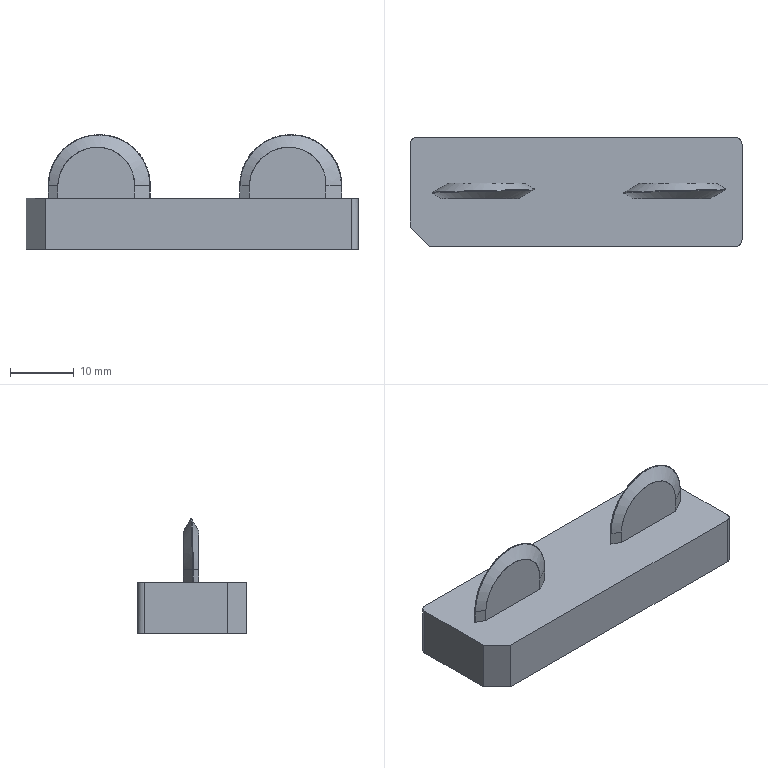NC program | PowerMill | posted with a generic post | part box 52 x 17 x 17.993 mm
Lines 1 to 1042 of 175197:
%
O0001
N104 ( POWERMILL CB  : 2026004.0)
N105 ( POST VER      : 2026.0.0.5161)
N106 ( OPTION FILE   : FANUC)
N107 ( OUTPUT WORKPLANE : WORLD)
N108 (  )
N109 ( TOOL LIST )
N110 (---------------------------------------)
N111 ( NO. | ID        | DIA.| TIP RAD|LENGTH)
N112 (---------------------------------------)
N113 (    1|D10C_1_1_1 |10.0 |  0.0   |73.44 )
N114 (    2|D4C_1_1    | 4.0 |  0.0   |65.16 )
N115 (    3|D10_1_1_1  |10.0 |  0.0   |73.16 )
N116 (    4|R1_1_1     | 2.0 |  1.0   | 64.4 )
N117 (   10|D3_1_1     | 3.0 |  0.0   |65.28 )
N118 (   13|TEXT_D4_1_1| 4.0 |  0.3   |65.24 )
N119 (---------------------------------------)
N120 (  )
N121 ( NUMBER OF TOOLPATHS: 9.0 )
N122 ( ESTIMATED PROGRAM DURATION: 0 HOURS 14 MIN 44 SEC)
N123 (  )
N124 G00 G21 G80 G40 G17
N125 G90
N126 G54
N127 G53 Z0.0
N128 (---------------)
N129 ( START TOOLPATH : 精公开粗01-扫面平行-D10C )
N130 (---------------)
N131 ( TOOL NO.    :1 )
N132 ( TOOL TYPE   : ENDMILL)
N133 ( TOOL ID     : D10C_1_1_1)
N134 ( TOOL DIA    : 10.0 LENGTH 73.44)
N135 T1
N136 M6
N137 S8000 M03
N138 G00 G90 X0.0 Y0.0
N139 G43 Z10.2 H1
N140
N141 G05 P10000 R4
N142 X33.8 Y11.3
N143 Z1.152
N144 G01 Z-0.048 F6000.0
N145 X28.8 F10000.0
N146 X-28.8
N147 Y5.65
N148 X28.8
N149 Y0.0
N150 X-28.8
N151 Y-5.65
N152 X28.8
N153 Y-11.3
N154 X-28.8
N155 X-33.8
N156 G00 Z10.2
N157 G05 P0
N158 (---------------)
N159 ( END TOOLPATH : 精公开粗01-扫面平行-D10C )
N160 (---------------)
N161 ( START TOOLPATH : 精公开粗01-外形偏置-D10C )
N162 (---------------)
N163 G00 X0.467 Y0.0 Z9.902
N164 G05 P10000 R4
N165 X-20.1146 Y16.575
N166 Z0.7059
N167 G01 Z-0.4941 F6000.0
N168 Y16.0475 F10000.0
N169 G03 X-15.3671 Y11.3 I4.7475 J0.0
N170 G01 X15.031
N171 X15.3555 Y5.6619
N172 X15.5488 Y5.6731
N173 X16.3222 Y5.6668
N174 X17.8691 Y5.5575
N175 X18.6425 Y5.4508
N176 X19.4159 Y5.2563
N177 X20.1894 Y4.9472
N178 X20.9628 Y4.4839
N179 X21.2604 Y4.2538
N180 X21.7362 Y3.8022
N181 X22.0145 Y3.4804
N182 X22.5239 Y2.707
N183 X22.8623 Y1.9336
N184 X23.0648 Y1.1601
N185 X23.1469 Y0.3867
N186 X23.1193 Y-0.3867
N187 X22.9748 Y-1.1601
N188 X22.7059 Y-1.9336
N189 X22.5097 Y-2.3365
N190 X22.2861 Y-2.707
N191 X21.7362 Y-3.4106
N192 X20.9628 Y-4.0912
N193 X20.7243 Y-4.2538
N194 X20.1894 Y-4.5543
N195 X19.4159 Y-4.8679
N196 X18.8482 Y-5.0273
N197 X17.8691 Y-5.1979
N198 X16.3222 Y-5.3576
N199 X15.5488 Y-5.3924
N200 X14.7754 Y-5.3899
N201 X13.2285 Y-5.2939
N202 X12.4551 Y-5.198
N203 X11.699 Y-5.0273
N204 X10.9083 Y-4.739
N205 X10.1348 Y-4.3084
N206 X9.3614 Y-3.6778
N207 X9.1718 Y-3.4804
N208 X8.5866 Y-2.707
N209 X8.1955 Y-1.9336
N210 X7.9426 Y-1.1601
N211 X7.8191 Y-0.3867
N212 X7.813 Y0.0303
N213 X3.1961 Y-0.0196
N214 G03 X3.8356 Y-3.4017 I9.825 J0.1062
N215 G01 X4.3225 Y-4.6838
N216 G02 X2.9383 Y-6.6901 I-1.3842 J-0.5257
N217 G01 X-2.0806 Y-6.6902
N218 G02 X-3.432 Y-4.7024 I0.0 J1.4533
N219 G01 X-2.9405 Y-3.4598
N220 G03 X-2.4579 Y-1.8025 I-8.6123 J3.4066
N221 G01 X-2.4294 Y-1.6543
N222 G03 X-2.7691 Y3.3599 I-9.6844 J1.8626
N223 G01 X-3.2133 Y4.677
N224 G02 X-1.7677 Y6.6901 I1.4456 J0.4875
N225 G01 X2.808
N226 G02 X4.2262 Y4.6814 I0.0 J-1.505
N227 G01 X3.7623 Y3.3756
N228 G03 X3.1961 Y-0.0196 I9.2588 J-3.289
N229 G01 X7.813 Y0.0303
N230 X7.8079 Y0.3867
N231 X7.9066 Y1.1601
N232 X8.1281 Y1.9336
N233 X8.4898 Y2.707
N234 X9.0292 Y3.4804
N235 X9.3614 Y3.8391
N236 X9.8321 Y4.2538
N237 X10.1348 Y4.4713
N238 X10.9083 Y4.9014
N239 X11.6817 Y5.1919
N240 X12.4551 Y5.3725
N241 X13.2285 Y5.4966
N242 X14.002 Y5.584
N243 X15.3555 Y5.6619
N244 X15.031 Y11.3
N245 X30.256
N246 G02 X31.256 Y10.3 I0.0 J-1.0
N247 G01 Y6.2153
N248 X26.256
N249 Y6.1307
N250 X26.1901 Y6.2308
N251 X26.167 Y6.2655
N252 X26.1436 Y6.3
N253 X26.256
N254 Y6.2153
N255 X31.256
N256 Y-6.1354
N257 X26.3408
N258 G02 X25.9821 I-0.1793 J0.0
N259 G02 X26.3408 I0.1794 J0.0
N260 G01 X31.256
N261 Y-10.3
N262 G02 X30.256 Y-11.3 I-1.0 J0.0
N263 G01 X-29.322
N264 G02 X-30.322 Y-10.3 I0.0 J1.0
N265 G01 Y10.3
N266 G02 X-29.322 Y11.3 I1.0 J0.0
N267 G01 X-25.2388
N268 Y6.3515
N269 G02 X-25.1309 Y6.2436 I0.0 J-0.1079
N270 G02 X-25.3467 I-0.1079 J0.0
N271 G02 X-25.2388 Y6.3515 I0.1079 J0.0
N272 G01 Y11.3
N273 X-15.3671
N274 X-15.0982 Y5.6473
N275 X-14.6148 Y5.6703
N276 X-13.8414 Y5.6695
N277 X-12.2945 Y5.5758
N278 X-11.5211 Y5.4789
N279 X-10.7477 Y5.3053
N280 X-9.9743 Y5.0224
N281 X-9.2008 Y4.5959
N282 X-8.7397 Y4.2538
N283 X-8.4274 Y3.9714
N284 X-7.9851 Y3.4804
N285 X-7.654 Y3.0059
N286 X-7.4764 Y2.707
N287 X-7.1374 Y1.9336
N288 X-6.9344 Y1.1601
N289 X-6.8536 Y0.3867
N290 X-6.8804 Y-0.3867
N291 X-7.0249 Y-1.1601
N292 X-7.2911 Y-1.9336
N293 X-7.654 Y-2.6161
N294 X-8.33 Y-3.4804
N295 X-9.2008 Y-4.2047
N296 X-9.9743 Y-4.6313
N297 X-10.7477 Y-4.9196
N298 X-11.1518 Y-5.0273
N299 X-12.2945 Y-5.2213
N300 X-13.8414 Y-5.3676
N301 X-14.6148 Y-5.3932
N302 X-15.3882 Y-5.3883
N303 X-16.9351 Y-5.2745
N304 X-17.7085 Y-5.1703
N305 X-18.3007 Y-5.0273
N306 X-19.2554 Y-4.6605
N307 X-19.9459 Y-4.2538
N308 X-20.8022 Y-3.5089
N309 X-21.0038 Y-3.2441
N310 X-25.1615 Y-6.1065
N311 X-25.1581 Y-6.112
N312 X-25.1552 Y-6.1179
N313 X-25.1337 Y-6.1686
N314 G02 X-25.2221 Y-6.2283 I-0.05 J-0.0213
N315 G01 X-25.2363 Y-6.2142
N316 X-25.2611 Y-6.1893
N317 X-25.2798 Y-6.1371
N318 X-25.2514 Y-6.0894
N319 X-25.203 Y-6.0795
N320 X-25.1615 Y-6.1065
N321 X-21.0038 Y-3.2441
N322 X-21.4128 Y-2.707
N323 X-21.5757 Y-2.4236
N324 X-21.8083 Y-1.9336
N325 X-22.0574 Y-1.1601
N326 X-22.1813 Y-0.3867
N327 X-22.1923 Y0.3867
N328 X-22.0932 Y1.1601
N329 X-21.8712 Y1.9336
N330 X-21.5757 Y2.584
N331 X-20.9712 Y3.4804
N332 X-20.8022 Y3.6702
N333 X-20.1679 Y4.2538
N334 X-19.2554 Y4.8241
N335 X-18.4819 Y5.1405
N336 X-17.7085 Y5.343
N337 X-16.9351 Y5.4724
N338 X-15.3882 Y5.6335
N339 X-15.0982 Y5.6473
N340 X-15.3671 Y11.3
N341 G00 Z3.3098
N342 G01 X-20.1146 Y16.575
N343 G00 Z0.3098
N344 G01 Z-0.8902 F6000.0
N345 Y16.0475 F10000.0
N346 G03 X-15.3671 Y11.3 I4.7475 J0.0
N347 G01 X14.5559
N348 X14.7754 Y5.8707
N349 X15.5488 Y5.9019
N350 X16.3222 Y5.8955
N351 X17.692 Y5.8007
N352 X18.6425 Y5.6777
N353 X19.4159 Y5.5428
N354 X20.1894 Y5.369
N355 X20.9628 Y5.0864
N356 X21.7362 Y4.6711
N357 X22.299 Y4.2538
N358 X22.5097 Y4.0648
N359 X23.0411 Y3.4804
N360 X23.2831 Y3.1445
N361 X23.5417 Y2.707
N362 X23.8766 Y1.9336
N363 X24.0565 Y1.2516
N364 X24.1504 Y0.3867
N365 X24.1217 Y-0.3867
N366 X24.0565 Y-0.8111
N367 X23.9729 Y-1.1601
N368 X23.7015 Y-1.9336
N369 X23.2831 Y-2.6992
N370 X22.6539 Y-3.4804
N371 X22.5097 Y-3.6199
N372 X21.7362 Y-4.2297
N373 X20.9628 Y-4.6486
N374 X20.1894 Y-4.9331
N375 X19.8327 Y-5.0273
N376 X18.6425 Y-5.2871
N377 X17.8691 Y-5.4178
N378 X16.3222 Y-5.5853
N379 X15.5488 Y-5.6207
N380 X14.7754 Y-5.6194
N381 X14.002 Y-5.5836
N382 X12.4551 Y-5.4231
N383 X10.9083 Y-5.1305
N384 X10.5494 Y-5.0273
N385 X10.1348 Y-4.8727
N386 X9.3614 Y-4.4858
N387 X9.0092 Y-4.2538
N388 X8.588 Y-3.9225
N389 X8.1409 Y-3.4804
N390 X7.8146 Y-3.0792
N391 X7.5656 Y-2.707
N392 X7.1758 Y-1.9336
N393 X6.9324 Y-1.1601
N394 X6.8121 Y-0.3867
N395 X6.8044 Y0.3867
N396 X6.9081 Y1.1601
N397 X7.0411 Y1.6716
N398 X7.1333 Y1.9336
N399 X7.4984 Y2.707
N400 X7.8146 Y3.1908
N401 X8.042 Y3.4804
N402 X8.588 Y4.036
N403 X8.8527 Y4.2538
N404 X9.3614 Y4.5993
N405 X10.1348 Y4.9913
N406 X10.9083 Y5.2519
N407 X12.4551 Y5.5906
N408 X13.2285 Y5.7174
N409 X14.7754 Y5.8707
N410 X14.5559 Y11.3
N411 X30.256
N412 G02 X31.256 Y10.3 I0.0 J-1.0
N413 G01 Y-10.3
N414 G02 X30.256 Y-11.3 I-1.0 J0.0
N415 G01 X-29.322
N416 G02 X-30.322 Y-10.3 I0.0 J1.0
N417 G01 Y10.3
N418 G02 X-29.322 Y11.3 I1.0 J0.0
N419 G01 X-15.6424
N420 X-15.3882 Y5.8625
N421 X-14.6148 Y5.8986
N422 X-13.8414 Y5.8987
N423 X-12.2945 Y5.7998
N424 X-11.5211 Y5.7026
N425 X-9.9743 Y5.4127
N426 X-9.2008 Y5.1556
N427 X-8.9067 Y5.0273
N428 X-8.4274 Y4.773
N429 X-7.7017 Y4.2538
N430 X-6.9595 Y3.4804
N431 X-6.4581 Y2.707
N432 X-6.1243 Y1.9336
N433 X-5.9279 Y1.1601
N434 X-5.8479 Y0.3867
N435 X-5.859 Y0.1083
N436 X-0.0971 Y-0.0337
N437 G03 X-0.4974 Y3.175 I-10.9069 J0.2687
N438 G01 X-0.7678 Y4.1414
N439 G02 X0.3038 Y5.554 I1.0716 J0.2999
N440 G01 X0.7376
N441 G02 X1.7888 Y4.1432 I0.0 J-1.0969
N442 G01 X1.504 Y3.1895
N443 G03 X1.5449 Y-3.2009 I10.4781 J-3.1283
N444 G01 X1.84 Y-4.145
N445 G02 X0.8041 Y-5.5541 I-1.0359 J-0.3237
N446 G01 X0.048
N447 G02 X-0.965 Y-4.148 I0.0 J1.068
N448 G01 X-0.6549 Y-3.2189
N449 G03 X-0.0971 Y-0.0337 I-10.3491 J3.4539
N450 G01 X-5.859 Y0.1083
N451 X-5.8788 Y-0.3867
N452 X-6.0256 Y-1.1601
N453 X-6.2972 Y-1.9336
N454 X-6.7221 Y-2.707
N455 X-6.8806 Y-2.9296
N456 X-7.3471 Y-3.4804
N457 X-7.654 Y-3.7709
N458 X-8.301 Y-4.2538
N459 X-9.2008 Y-4.7197
N460 X-10.1694 Y-5.0273
N461 X-11.5211 Y-5.3172
N462 X-12.2945 Y-5.4437
N463 X-13.8414 Y-5.5955
N464 X-14.6148 Y-5.6227
N465 X-15.3882 Y-5.617
N466 X-16.1617 Y-5.5733
N467 X-17.7085 Y-5.3967
N468 X-18.4819 Y-5.2618
N469 X-19.2554 Y-5.0864
N470 X-20.0288 Y-4.8006
N471 X-20.8022 Y-4.3836
N472 X-20.9907 Y-4.2538
N473 X-21.5757 Y-3.7721
N474 X-21.8595 Y-3.4804
N475 X-22.3491 Y-2.8413
N476 X-22.8229 Y-1.9336
N477 X-23.0672 Y-1.1601
N478 X-23.1871 Y-0.3867
N479 X-23.1952 Y0.3867
N480 X-23.1225 Y1.0043
N481 X-22.868 Y1.9336
N482 X-22.5013 Y2.707
N483 X-22.3491 Y2.9528
N484 X-21.955 Y3.4804
N485 X-21.5757 Y3.8827
N486 X-21.1473 Y4.2538
N487 X-20.8022 Y4.4978
N488 X-20.0288 Y4.9199
N489 X-19.2554 Y5.2065
N490 X-17.7085 Y5.5622
N491 X-16.9351 Y5.692
N492 X-15.3882 Y5.8625
N493 X-15.6424 Y11.3
N494 X-15.3671
N495 G00 Z2.9138
N496 G01 X-20.1146 Y16.575
N497 G00 Z-0.0862
N498 G01 Z-1.2862 F6000.0
N499 Y16.0475 F10000.0
N500 G03 X-15.3671 Y11.3 I4.7475 J0.0
N501 G01 X0.5041
N502 Y4.8801
N503 G02 X0.6277 Y4.7565 I0.0 J-0.1236
N504 G02 X0.3805 I-0.1236 J0.0
N505 G02 X0.5041 Y4.8801 I0.1236 J0.0
N506 G01 Y11.3
N507 X15.593
N508 X15.5488 Y6.1308
N509 X16.3222 Y6.1242
N510 X17.0957 Y6.0803
N511 X17.8691 Y6.0037
N512 X18.6425 Y5.8968
N513 X19.4159 Y5.7589
N514 X20.9628 Y5.3876
N515 X21.7362 Y5.1002
N516 X22.5097 Y4.6708
N517 X23.0588 Y4.2538
N518 X23.2831 Y4.0501
N519 X23.7918 Y3.4804
N520 X24.0565 Y3.1
N521 X24.2866 Y2.707
N522 X24.6153 Y1.9336
N523 X24.8098 Y1.1601
N524 X24.8845 Y0.3867
N525 X24.8492 Y-0.3867
N526 X24.7033 Y-1.1601
N527 X24.4279 Y-1.9336
N528 X24.0565 Y-2.6181
N529 X23.3714 Y-3.4804
N530 X22.5097 Y-4.19
N531 X21.7362 Y-4.6238
N532 X20.9628 Y-4.9128
N533 X20.1894 Y-5.1364
N534 X18.6425 Y-5.5037
N535 X17.8691 Y-5.6378
N536 X16.4895 Y-5.8007
N537 X15.5488 Y-5.8491
N538 X14.7754 Y-5.8488
N539 X13.8287 Y-5.8007
N540 X12.4551 Y-5.6423
N541 X11.6817 Y-5.5096
N542 X10.9083 Y-5.341
N543 X9.7248 Y-5.0273
N544 X9.3614 Y-4.8868
N545 X8.588 Y-4.4856
N546 X8.2414 Y-4.2538
N547 X7.8146 Y-3.9102
N548 X7.3887 Y-3.4804
N549 X7.0411 Y-3.0456
N550 X6.82 Y-2.707
N551 X6.435 Y-1.9336
N552 X6.1959 Y-1.1601
N553 X6.0782 Y-0.3867
N554 X6.0729 Y0.3867
N555 X6.1795 Y1.1601
N556 X6.2677 Y1.5167
N557 X6.4073 Y1.9336
N558 X6.775 Y2.707
N559 X7.0411 Y3.1186
N560 X7.3225 Y3.4804
N561 X7.8146 Y3.9848
N562 X8.1387 Y4.2538
N563 X8.588 Y4.5623
N564 X9.3614 Y4.967
N565 X10.1348 Y5.2377
N566 X10.9083 Y5.4512
N567 X12.4551 Y5.8088
N568 X13.2285 Y5.9382
N569 X14.002 Y6.0343
N570 X14.7754 Y6.0994
N571 X15.5488 Y6.1308
N572 X15.593 Y11.3
N573 X30.256
N574 G02 X31.256 Y10.3 I0.0 J-1.0
N575 G01 Y-10.3
N576 G02 X30.256 Y-11.3 I-1.0 J0.0
N577 G01 X0.4352
N578 Y-5.453
N579 G02 X-0.133 Y-4.8848 I0.0 J0.5682
N580 G02 X1.0034 I0.5682 J0.0
N581 G02 X0.4352 Y-5.453 I-0.5682 J0.0
N582 G01 Y-11.3
N583 X-29.322
N584 G02 X-30.322 Y-10.3 I0.0 J1.0
N585 G01 Y10.3
N586 G02 X-29.322 Y11.3 I1.0 J0.0
N587 G01 X-15.5396
N588 X-15.2916 Y6.0948
N589 X-14.6148 Y6.127
N590 X-13.8414 Y6.1279
N591 X-12.2945 Y6.0238
N592 X-10.8029 Y5.8007
N593 X-9.2008 Y5.4327
N594 X-8.4274 Y5.1722
N595 X-8.1115 Y5.0273
N596 X-7.654 Y4.7743
N597 X-6.9421 Y4.2538
N598 X-6.2084 Y3.4804
N599 X-5.7134 Y2.707
N600 X-5.3845 Y1.9336
N601 X-5.1902 Y1.1601
N602 X-5.1155 Y0.3867
N603 X-5.1484 Y-0.3867
N604 X-5.2966 Y-1.1601
N605 X-5.5722 Y-1.9336
N606 X-5.999 Y-2.707
N607 X-6.629 Y-3.4804
N608 X-6.8806 Y-3.7203
N609 X-7.59 Y-4.2538
N610 X-8.4274 Y-4.6966
N611 X-9.2008 Y-4.9635
N612 X-9.9743 Y-5.1807
N613 X-11.5211 Y-5.535
N614 X-12.2945 Y-5.6643
N615 X-13.5035 Y-5.8007
N616 X-14.6148 Y-5.8521
N617 X-15.3882 Y-5.8454
N618 X-16.1781 Y-5.8007
N619 X-16.9351 Y-5.7241
N620 X-18.4819 Y-5.4772
N621 X-20.0288 Y-5.1053
N622 X-20.8022 Y-4.815
N623 X-21.5757 Y-4.3819
N624 X-21.7585 Y-4.2538
N625 X-22.3491 Y-3.7557
N626 X-22.6127 Y-3.4804
N627 X-23.1225 Y-2.8001
N628 X-23.5635 Y-1.9336
N629 X-23.8037 Y-1.1601
N630 X-23.9209 Y-0.3867
N631 X-23.9266 Y0.3867
N632 X-23.8214 Y1.1601
N633 X-23.5932 Y1.9336
N634 X-23.2246 Y2.707
N635 X-22.6765 Y3.4804
N636 X-22.3491 Y3.8297
N637 X-21.8617 Y4.2538
N638 X-21.5757 Y4.4577
N639 X-20.8022 Y4.8928
N640 X-20.4937 Y5.0273
N641 X-20.0288 Y5.1868
N642 X-19.2554 Y5.4074
N643 X-17.7085 Y5.7785
N644 X-16.9351 Y5.9117
N645 X-15.3882 Y6.0902
N646 X-15.2916 Y6.0948
N647 X-15.5396 Y11.3
N648 X-15.3671
N649 G00 Z2.5177
N650 G01 X-20.1146 Y16.575
N651 G00 Z-0.4823
N652 G01 Z-1.6823 F6000.0
N653 Y16.0475 F10000.0
N654 G03 X-15.3671 Y11.3 I4.7475 J0.0
N655 G01 X-15.3425
N656 X-15.0982 Y6.3316
N657 X-14.6148 Y6.3554
N658 X-13.8414 Y6.3571
N659 X-13.068 Y6.3179
N660 X-12.2945 Y6.2479
N661 X-11.5211 Y6.1431
N662 X-10.7477 Y6.006
N663 X-9.831 Y5.8007
N664 X-8.4274 Y5.4065
N665 X-7.654 Y5.1143
N666 X-6.8806 Y4.6743
N667 X-6.3346 Y4.2538
N668 X-6.1071 Y4.0428
N669 X-5.6121 Y3.4804
N670 X-5.3337 Y3.0782
N671 X-5.1205 Y2.707
N672 X-4.7961 Y1.9336
N673 X-4.6036 Y1.1601
N674 X-4.5321 Y0.3867
N675 X-4.5603 Y-0.3229
N676 X-4.7171 Y-1.1601
N677 X-4.996 Y-1.9336
N678 X-5.4252 Y-2.707
N679 X-6.0579 Y-3.4804
N680 X-6.8806 Y-4.1622
N681 X-7.654 Y-4.6039
N682 X-8.4274 Y-4.9042
N683 X-9.2008 Y-5.1573
N684 X-10.7477 Y-5.581
N685 X-11.7985 Y-5.8007
N686 X-13.068 Y-5.9842
N687 X-13.8414 Y-6.0513
N688 X-14.6148 Y-6.0815
N689 X-15.3882 Y-6.0739
N690 X-16.1617 Y-6.0297
N691 X-16.9351 Y-5.9488
N692 X-17.7085 Y-5.8347
N693 X-19.2554 Y-5.5128
N694 X-20.8022 Y-5.0705
N695 X-21.5757 Y-4.748
N696 X-22.3491 Y-4.2709
N697 X-23.1225 Y-3.5824
N698 X-23.7781 Y-2.707
N699 X-24.1583 Y-1.9336
N700 X-24.394 Y-1.1601
N701 X-24.5097 Y-0.3867
N702 X-24.512 Y0.3867
N703 X-24.404 Y1.1601
N704 X-24.1729 Y1.9336
N705 X-23.8025 Y2.707
N706 X-23.2519 Y3.4804
N707 X-23.1225 Y3.6245
N708 X-22.43 Y4.2538
N709 X-21.5757 Y4.7939
N710 X-21.0548 Y5.0273
N711 X-20.0288 Y5.3779
N712 X-18.5515 Y5.8007
N713 X-17.7085 Y5.991
N714 X-16.9351 Y6.1314
N715 X-16.1617 Y6.241
N716 X-15.3882 Y6.3174
N717 X-15.0982 Y6.3316
N718 X-15.3425 Y11.3
N719 X0.5926
N720 Y5.2752
N721 G02 X0.7661 Y5.1017 I0.0 J-0.1735
N722 G02 X0.419 I-0.1735 J0.0
N723 G02 X0.5926 Y5.2752 I0.1736 J0.0
N724 G01 Y11.3
N725 X15.0567
N726 X15.2588 Y6.3479
N727 X15.5488 Y6.3597
N728 X16.3222 Y6.3529
N729 X17.0957 Y6.3082
N730 X17.8691 Y6.2275
N731 X18.6425 Y6.1159
N732 X19.4159 Y5.9719
N733 X20.1693 Y5.8007
N734 X21.7362 Y5.3538
N735 X22.5097 Y5.0353
N736 X23.2831 Y4.5592
N737 X23.6659 Y4.2538
N738 X24.0565 Y3.8738
N739 X24.3894 Y3.4804
N740 X24.8299 Y2.796
N741 X25.2042 Y1.9336
N742 X25.3956 Y1.1601
N743 X25.4675 Y0.3867
N744 X25.4323 Y-0.3867
N745 X25.2829 Y-1.1601
N746 X25.0047 Y-1.9336
N747 X24.8299 Y-2.2856
N748 X24.5748 Y-2.707
N749 X24.0565 Y-3.3609
N750 X23.2831 Y-4.0449
N751 X22.9827 Y-4.2538
N752 X22.5097 Y-4.5243
N753 X21.7362 Y-4.8479
N754 X20.9628 Y-5.1069
N755 X19.4159 Y-5.5432
N756 X18.2013 Y-5.8007
N757 X17.0957 Y-5.9663
N758 X16.3222 Y-6.0407
N759 X15.5488 Y-6.0774
N760 X14.7754 Y-6.0783
N761 X14.002 Y-6.04
N762 X13.2285 Y-5.9673
N763 X12.0936 Y-5.8007
N764 X10.9083 Y-5.5514
N765 X9.3614 Y-5.1231
N766 X8.588 Y-4.8284
N767 X7.8146 Y-4.3855
N768 X7.628 Y-4.2538
N769 X7.0411 Y-3.7518
N770 X6.7844 Y-3.4804
N771 X6.2677 Y-2.7817
N772 X5.8439 Y-1.9336
N773 X5.6042 Y-1.1601
N774 X5.4943 Y-0.4254
N775 X5.4884 Y0.3867
N776 X5.5953 Y1.1601
N777 X5.8258 Y1.9336
N778 X6.1978 Y2.707
N779 X6.7498 Y3.4804
N780 X7.0411 Y3.7941
N781 X7.5693 Y4.2538
N782 X7.8146 Y4.43
N783 X8.588 Y4.8744
N784 X8.9431 Y5.0273
N785 X10.1348 Y5.4304
N786 X11.447 Y5.8007
N787 X12.4551 Y6.0259
N788 X13.2285 Y6.159
N789 X14.002 Y6.2594
N790 X14.7754 Y6.3281
N791 X15.2588 Y6.3479
N792 X15.0567 Y11.3
N793 X30.256
N794 G02 X31.256 Y10.3 I0.0 J-1.0
N795 G01 Y-10.3
N796 G02 X30.256 Y-11.3 I-1.0 J0.0
N797 G01 X0.4138
N798 Y-5.4387
N799 G02 X0.1351 Y-5.16 I0.0 J0.2787
N800 G02 X0.6924 I0.2787 J0.0
N801 G02 X0.4138 Y-5.4387 I-0.2786 J0.0
N802 G01 Y-11.3
N803 X-29.322
N804 G02 X-30.322 Y-10.3 I0.0 J1.0
N805 G01 Y10.3
N806 G02 X-29.322 Y11.3 I1.0 J0.0
N807 G01 X-15.3671
N808 G00 Z2.1216
N809 G01 X-20.1146 Y16.575
N810 G00 Z-0.8784
N811 G01 Z-2.0784 F6000.0
N812 Y16.0475 F10000.0
N813 G03 X-15.3671 Y11.3 I4.7475 J0.0
N814 G01 X-14.9014
N815 Y6.5741
N816 X-13.5162
N817 X-12.2945 Y6.4719
N818 X-11.5211 Y6.3624
N819 X-10.7477 Y6.2185
N820 X-9.9743 Y6.042
N821 X-9.0816 Y5.8007
N822 X-7.654 Y5.3363
N823 X-6.9373 Y5.0273
N824 X-6.1071 Y4.4916
N825 X-5.8182 Y4.2538
N826 X-5.3337 Y3.7645
N827 X-5.1018 Y3.4804
N828 X-4.616 Y2.707
N829 X-4.2937 Y1.9336
N830 X-4.1048 Y1.1601
N831 X-4.036 Y0.3867
N832 X-4.0729 Y-0.3867
N833 X-4.2247 Y-1.1601
N834 X-4.5066 Y-1.9336
N835 X-4.9378 Y-2.707
N836 X-5.3337 Y-3.2209
N837 X-5.5741 Y-3.4804
N838 X-6.1071 Y-3.9512
N839 X-6.5345 Y-4.2538
N840 X-6.8806 Y-4.4568
N841 X-7.654 Y-4.7987
N842 X-8.4274 Y-5.0854
N843 X-9.9743 Y-5.5853
N844 X-10.7861 Y-5.8007
N845 X-11.5211 Y-5.9647
N846 X-12.2945 Y-6.1055
N847 X-13.068 Y-6.2106
N848 X-13.8414 Y-6.2793
N849 X-14.6148 Y-6.3085
N850 X-15.3882 Y-6.3023
N851 X-16.1617 Y-6.2563
N852 X-16.9351 Y-6.1732
N853 X-17.7085 Y-6.0537
N854 X-18.9165 Y-5.8007
N855 X-20.0288 Y-5.5042
N856 X-21.4817 Y-5.0273
N857 X-22.3491 Y-4.6177
N858 X-22.8897 Y-4.2538
N859 X-23.1225 Y-4.0699
N860 X-23.7239 Y-3.4804
N861 X-23.8959 Y-3.2706
N862 X-24.2815 Y-2.707
N863 X-24.6579 Y-1.9336
N864 X-24.8924 Y-1.1601
N865 X-25.004 Y-0.3867
N866 X-25.003 Y0.3867
N867 X-24.8933 Y1.1601
N868 X-24.6628 Y1.9336
N869 X-24.2871 Y2.707
N870 X-23.8959 Y3.2834
N871 X-23.7351 Y3.4804
N872 X-23.1225 Y4.0836
N873 X-22.9095 Y4.2538
N874 X-22.3491 Y4.6322
N875 X-21.5757 Y5.0091
N876 X-20.0288 Y5.5674
N877 X-18.4819 Y6.0218
N878 X-17.7085 Y6.2036
N879 X-16.9351 Y6.3512
N880 X-16.1617 Y6.466
N881 X-14.9014 Y6.5741
N882 Y11.3
N883 X0.5813
N884 Y6.8
N885 Y11.3
N886 X15.076
N887 X15.0985 Y6.5741
N888 X16.3222 Y6.5799
N889 X17.0957 Y6.5359
N890 X17.8691 Y6.452
N891 X18.6425 Y6.335
N892 X19.4159 Y6.184
N893 X20.9168 Y5.8007
N894 X22.5097 Y5.2762
N895 X23.2831 Y4.9054
N896 X24.0565 Y4.3612
N897 X24.8299 Y3.5673
N898 X25.3841 Y2.707
N899 X25.6034 Y2.2192
N900 X25.706 Y1.9336
N901 X25.8949 Y1.1601
N902 X25.9651 Y0.3867
N903 X25.9279 Y-0.3867
N904 X25.7753 Y-1.1601
N905 X25.4949 Y-1.9336
N906 X25.0623 Y-2.707
N907 X24.8299 Y-3.0244
N908 X24.4259 Y-3.4804
N909 X24.0565 Y-3.8172
N910 X23.2831 Y-4.3649
N911 X22.5097 Y-4.7353
N912 X21.7319 Y-5.0273
N913 X20.1894 Y-5.5372
N914 X19.215 Y-5.8007
N915 X17.8691 Y-6.0776
N916 X17.0957 Y-6.1914
N917 X16.3222 Y-6.2685
N918 X15.5488 Y-6.3058
N919 X14.7754 Y-6.3077
N920 X14.002 Y-6.2689
N921 X13.2285 Y-6.1921
N922 X12.4551 Y-6.0808
N923 X10.9083 Y-5.7612
N924 X10.1348 Y-5.5504
N925 X8.5188 Y-5.0273
N926 X7.8146 Y-4.7099
N927 X7.1105 Y-4.2538
N928 X6.2761 Y-3.4804
N929 X5.7188 Y-2.707
N930 X5.4943 Y-2.2841
N931 X5.3426 Y-1.9336
N932 X5.1076 Y-1.1601
N933 X4.9979 Y-0.3867
N934 X4.9955 Y0.3867
N935 X5.105 Y1.1601
N936 X5.3375 Y1.9336
N937 X5.4943 Y2.297
N938 X5.7113 Y2.707
N939 X6.2677 Y3.4826
N940 X7.0411 Y4.2161
N941 X7.8146 Y4.7254
N942 X8.4709 Y5.0273
N943 X10.1348 Y5.6215
N944 X11.6817 Y6.0651
N945 X12.4551 Y6.2392
N946 X13.2285 Y6.3805
N947 X14.002 Y6.485
N948 X15.0985 Y6.5741
N949 X15.076 Y11.3
N950 X30.256
N951 G02 X31.256 Y10.3 I0.0 J-1.0
N952 G01 Y-10.3
N953 G02 X30.256 Y-11.3 I-1.0 J0.0
N954 G01 X0.3753
N955 Y-6.8
N956 Y-11.3
N957 X-29.322
N958 G02 X-30.322 Y-10.3 I0.0 J1.0
N959 G01 Y10.3
N960 G02 X-29.322 Y11.3 I1.0 J0.0
N961 G01 X-15.3671
N962 G00 Z1.7255
N963 G01 X-20.1146 Y16.575
N964 G00 Z-1.2745
N965 G01 Z-2.4745 F6000.0
N966 Y16.0475 F10000.0
N967 G03 X-15.3671 Y11.3 I4.7475 J0.0
N968 G01 X0.5867
N969 Y6.8
N970 Y11.3
N971 X15.951
N972 X15.9355 Y6.6531
N973 X17.8691 Y6.6467
N974 X18.521 Y6.5741
N975 X19.4159 Y6.396
N976 X20.9628 Y5.981
N977 X22.5097 Y5.4551
N978 X23.2831 Y5.1451
N979 X23.5197 Y5.0273
N980 X24.0565 Y4.7015
N981 X24.6236 Y4.2538
N982 X24.8299 Y4.0586
N983 X25.3347 Y3.4804
N984 X25.6034 Y3.0853
N985 X25.8168 Y2.707
N986 X26.1349 Y1.9336
N987 X26.3214 Y1.1601
N988 X26.3895 Y0.3867
N989 X26.3516 Y-0.3867
N990 X26.197 Y-1.1601
N991 X25.9139 Y-1.9336
N992 X25.4784 Y-2.707
N993 X24.8396 Y-3.4804
N994 X24.0565 Y-4.1331
N995 X23.2831 Y-4.5773
N996 X22.5097 Y-4.9024
N997 X20.9628 Y-5.4812
N998 X19.9619 Y-5.8007
N999 X18.6425 Y-6.1423
N1000 X17.8691 Y-6.2935
N1001 X17.0957 Y-6.3539
N1002 X13.2285 Y-6.3542
N1003 X12.4551 Y-6.2947
N1004 X11.6817 Y-6.1489
N1005 X10.9083 Y-5.9659
N1006 X10.1348 Y-5.7496
N1007 X9.3614 Y-5.5016
N1008 X7.8146 Y-4.9331
N1009 X7.0411 Y-4.5215
N1010 X6.6593 Y-4.2538
N1011 X6.2677 Y-3.9237
N1012 X5.8381 Y-3.4804
N1013 X5.4943 Y-3.0358
N1014 X5.2834 Y-2.707
N1015 X4.9102 Y-1.9336
N1016 X4.7208 Y-1.3386
N1017 X4.5685 Y-0.3867
N1018 X4.5695 Y0.3867
N1019 X4.6812 Y1.1601
N1020 X4.9157 Y1.9336
N1021 X5.2919 Y2.707
N1022 X5.4943 Y3.0221
N1023 X5.8508 Y3.4804
N1024 X6.2677 Y3.9115
N1025 X6.674 Y4.2538
N1026 X7.0411 Y4.5109
N1027 X7.8146 Y4.9222
N1028 X8.588 Y5.2386
N1029 X10.1348 Y5.808
N1030 X11.6817 Y6.271
N1031 X13.0803 Y6.5741
N1032 X14.002 Y6.6596
N1033 X15.9355 Y6.6531
N1034 X15.951 Y11.3
N1035 X30.256
N1036 G02 X31.256 Y10.3 I0.0 J-1.0
N1037 G01 Y-10.3
N1038 G02 X30.256 Y-11.3 I-1.0 J0.0
N1039 G01 X0.3466
N1040 Y-6.8
N1041 Y-11.3
N1042 X-29.322
N1043 G02 X-30.322 Y-10.3 I0.0 J1.0
N1044 G01 Y10.3
N1045 G02 X-29.322 Y11.3 I1.0 J0.0
N1046 G01 X-16.1676
N1047 X-16.1617 Y6.6504
N1048 X-12.2945 Y6.6554
N1049 X-11.5211 Y6.5802
N1050 X-10.7477 Y6.431
N1051 X-9.9743 Y6.2462
N1052 X-8.4697 Y5.8007
N1053 X-6.8806 Y5.2173
N1054 X-6.4802 Y5.0273
N1055 X-6.1071 Y4.8103
N1056 X-5.3756 Y4.2538
N1057 X-4.6653 Y3.4804
N1058 X-4.1832 Y2.707
N1059 X-3.864 Y1.9336
N1060 X-3.6772 Y1.1601
N1061 X-3.6094 Y0.3867
N1062 X-3.6504 Y-0.3867
N1063 X-3.7868 Y-1.0973
N1064 X-4.0855 Y-1.9336
N1065 X-4.5222 Y-2.707
N1066 X-5.1607 Y-3.4804
N1067 X-5.3337 Y-3.6448
N1068 X-6.1257 Y-4.2538
N1069 X-6.8806 Y-4.6495
N1070 X-7.654 Y-4.9663
N1071 X-9.2008 Y-5.5379
N1072 X-10.038 Y-5.8007
N1073 X-11.5211 Y-6.1793
N1074 X-12.2945 Y-6.314
N1075 X-13.068 Y-6.3548
N1076 X-16.9351 Y-6.3497
N1077 X-17.7085 Y-6.2688
N1078 X-18.4819 Y-6.11
N1079 X-19.2554 Y-5.9204
N1080 X-20.8022 Y-5.448
N1081 X-21.9534 Y-5.0273
N1082 X-22.3491 Y-4.8594
N1083 X-23.1225 Y-4.413
N1084 X-23.3407 Y-4.2538
N1085 X-23.8959 Y-3.7668
N1086 X-24.1631 Y-3.4804
N1087 X-24.6694 Y-2.7843
N1088 X-25.088 Y-1.9336
N1089 X-25.3204 Y-1.1601
N1090 X-25.4315 Y-0.3867
N1091 X-25.4305 Y0.3867
N1092 X-25.3188 Y1.1601
N1093 X-25.0824 Y1.9336
N1094 X-24.7082 Y2.707
N1095 X-24.1512 Y3.4804
N1096 X-23.8959 Y3.7545
N1097 X-23.3243 Y4.2538
N1098 X-23.1225 Y4.4014
N1099 X-22.3491 Y4.8485
N1100 X-20.8022 Y5.4746
N1101 X-19.2554 Y6.0067
N1102 X-17.7085 Y6.4162
N1103 X-16.9351 Y6.5719
N1104 X-16.1617 Y6.6504
N1105 X-16.1676 Y11.3
N1106 X-15.3671
N1107 G00 Z1.3294
N1108 G01 X-20.1146 Y16.575
N1109 G00 Z-1.6706
N1110 G01 Z-2.8706 F6000.0
N1111 Y16.0475 F10000.0
N1112 G03 X-15.3671 Y11.3 I4.7475 J0.0
N1113 G01 X0.6002
N1114 Y6.8
N1115 Y11.3
N1116 X30.256
N1117 G02 X31.256 Y10.3 I0.0 J-1.0
N1118 G01 Y0.9644
N1119 X26.7445 Y0.5801
N1120 X26.761 Y0.3867
N1121 X26.7205 Y-0.3867
N1122 X26.5627 Y-1.1601
N1123 X26.2787 Y-1.9336
N1124 X25.8426 Y-2.707
N1125 X25.6034 Y-3.0304
N1126 X25.2001 Y-3.4804
N1127 X24.8299 Y-3.8176
N1128 X24.2304 Y-4.2538
N1129 X23.2831 Y-4.7333
N1130 X21.7362 Y-5.3738
N1131 X20.5727 Y-5.8007
N1132 X19.4159 Y-6.1555
N1133 X18.6425 Y-6.3102
N1134 X17.8691 Y-6.3548
N1135 X12.4551
N1136 X11.6817 Y-6.3159
N1137 X10.9083 Y-6.1697
N1138 X9.3614 Y-5.6879
N1139 X7.6352 Y-5.0273